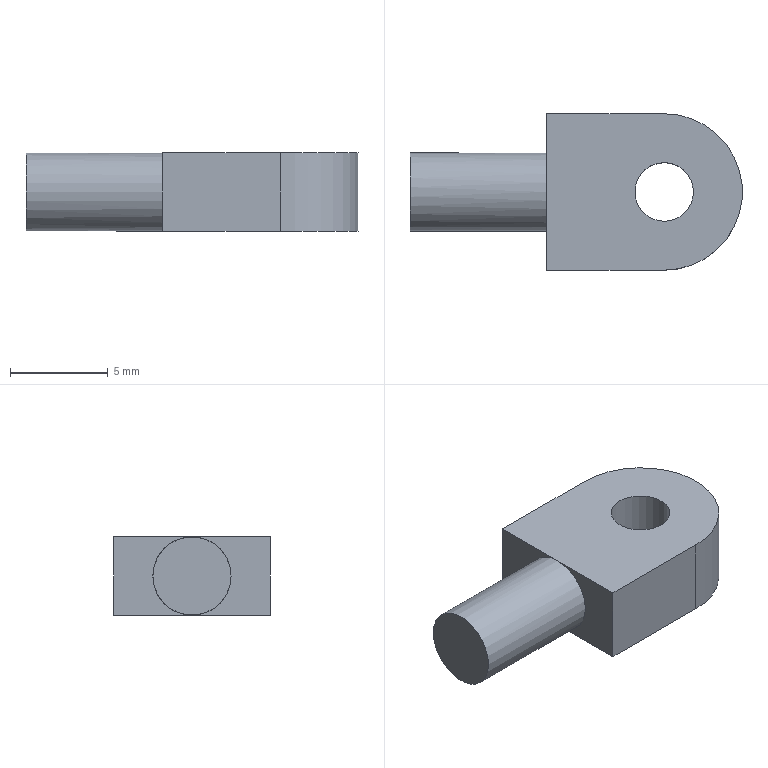Part | STEP file | 1-53.4 | 1 solid | 10 faces | box 17 x 8 x 4 mm | volume 352.221 mm3 | plane 7 | cylinder 3 | commonest cylinder face diameters 3 x1 4 x1 8 x1
STEP:
#1=CARTESIAN_POINT('',(0.,0.,0.));
#2=DIRECTION('',(0.,0.,1.));
#3=DIRECTION('',(1.,0.,0.));
#4=AXIS2_PLACEMENT_3D('',#1,#2,#3);
#5=CARTESIAN_POINT('',(0.,-4.,-2.));
#6=VERTEX_POINT('',#5);
#7=CARTESIAN_POINT('',(0.,4.,-2.));
#8=VERTEX_POINT('',#7);
#9=CARTESIAN_POINT('',(0.,0.,-2.));
#10=DIRECTION('',(0.,0.,1.));
#11=DIRECTION('',(0.,-1.,0.));
#12=AXIS2_PLACEMENT_3D('',#9,#10,#11);
#13=CIRCLE('',#12,4.);
#14=CARTESIAN_POINT('',(-1.,1.,-2.));
#15=DIRECTION('',(0.,0.,1.));
#16=DIRECTION('',(0.,1.,0.));
#17=AXIS2_PLACEMENT_3D('',#14,#15,#16);
#18=PLANE('',#17);
#19=CARTESIAN_POINT('',(-1.,-1.));
#20=DIRECTION('',(-1.,0.));
#21=AXIS2_PLACEMENT_2D('',#19,#20);
#22=CIRCLE('',#21,4.);
#23=(GEOMETRIC_REPRESENTATION_CONTEXT(2)PARAMETRIC_REPRESENTATION_CONTEXT()REPRESENTATION_CONTEXT('',''));
#24=DEFINITIONAL_REPRESENTATION('',(#22),#23);
#25=PCURVE('',#18,#24);
#26=CARTESIAN_POINT('',(0.,0.,-2.));
#27=DIRECTION('',(0.,0.,1.));
#28=DIRECTION('',(0.,-1.,0.));
#29=AXIS2_PLACEMENT_3D('',#26,#27,#28);
#30=CYLINDRICAL_SURFACE('',#29,4.);
#31=CARTESIAN_POINT('',(0.,0.));
#32=DIRECTION('',(1.,0.));
#33=VECTOR('',#32,1.);
#34=LINE('',#31,#33);
#35=(GEOMETRIC_REPRESENTATION_CONTEXT(2)PARAMETRIC_REPRESENTATION_CONTEXT()REPRESENTATION_CONTEXT('',''));
#36=DEFINITIONAL_REPRESENTATION('',(#34),#35);
#37=PCURVE('',#30,#36);
#38=SURFACE_CURVE('',#13,(#25,#37),.PCURVE_S1.);
#39=EDGE_CURVE('',#6,#8,#38,.T.);
#40=ORIENTED_EDGE('',*,*,#39,.T.);
#41=CARTESIAN_POINT('',(-6.,4.,-2.));
#42=VERTEX_POINT('',#41);
#43=CARTESIAN_POINT('',(0.,4.,-2.));
#44=DIRECTION('',(-1.,0.,0.));
#45=VECTOR('',#44,1.);
#46=LINE('',#43,#45);
#47=CARTESIAN_POINT('',(3.,-1.));
#48=DIRECTION('',(0.,1.));
#49=VECTOR('',#48,1.);
#50=LINE('',#47,#49);
#51=(GEOMETRIC_REPRESENTATION_CONTEXT(2)PARAMETRIC_REPRESENTATION_CONTEXT()REPRESENTATION_CONTEXT('',''));
#52=DEFINITIONAL_REPRESENTATION('',(#50),#51);
#53=PCURVE('',#18,#52);
#54=CARTESIAN_POINT('',(-3.,4.,0.));
#55=DIRECTION('',(0.,1.,0.));
#56=DIRECTION('',(-1.,0.,0.));
#57=AXIS2_PLACEMENT_3D('',#54,#55,#56);
#58=PLANE('',#57);
#59=CARTESIAN_POINT('',(-3.,-2.));
#60=DIRECTION('',(1.,0.));
#61=VECTOR('',#60,1.);
#62=LINE('',#59,#61);
#63=(GEOMETRIC_REPRESENTATION_CONTEXT(2)PARAMETRIC_REPRESENTATION_CONTEXT()REPRESENTATION_CONTEXT('',''));
#64=DEFINITIONAL_REPRESENTATION('',(#62),#63);
#65=PCURVE('',#58,#64);
#66=SURFACE_CURVE('',#46,(#53,#65),.PCURVE_S1.);
#67=EDGE_CURVE('',#8,#42,#66,.T.);
#68=ORIENTED_EDGE('',*,*,#67,.T.);
#69=CARTESIAN_POINT('',(-6.,0.,-2.));
#70=VERTEX_POINT('',#69);
#71=CARTESIAN_POINT('',(-6.,4.,-2.));
#72=DIRECTION('',(0.,-1.,0.));
#73=VECTOR('',#72,1.);
#74=LINE('',#71,#73);
#75=CARTESIAN_POINT('',(3.,5.));
#76=DIRECTION('',(-1.,0.));
#77=VECTOR('',#76,1.);
#78=LINE('',#75,#77);
#79=(GEOMETRIC_REPRESENTATION_CONTEXT(2)PARAMETRIC_REPRESENTATION_CONTEXT()REPRESENTATION_CONTEXT('',''));
#80=DEFINITIONAL_REPRESENTATION('',(#78),#79);
#81=PCURVE('',#18,#80);
#82=CARTESIAN_POINT('',(-6.,0.,0.));
#83=DIRECTION('',(-1.,0.,0.));
#84=DIRECTION('',(0.,-1.,0.));
#85=AXIS2_PLACEMENT_3D('',#82,#83,#84);
#86=PLANE('',#85);
#87=CARTESIAN_POINT('',(-4.,-2.));
#88=DIRECTION('',(1.,0.));
#89=VECTOR('',#88,1.);
#90=LINE('',#87,#89);
#91=(GEOMETRIC_REPRESENTATION_CONTEXT(2)PARAMETRIC_REPRESENTATION_CONTEXT()REPRESENTATION_CONTEXT('',''));
#92=DEFINITIONAL_REPRESENTATION('',(#90),#91);
#93=PCURVE('',#86,#92);
#94=SURFACE_CURVE('',#74,(#81,#93),.PCURVE_S1.);
#95=EDGE_CURVE('',#42,#70,#94,.T.);
#96=ORIENTED_EDGE('',*,*,#95,.T.);
#97=CARTESIAN_POINT('',(-6.,-4.,-2.));
#98=VERTEX_POINT('',#97);
#99=CARTESIAN_POINT('',(-6.,0.,-2.));
#100=DIRECTION('',(0.,-1.,0.));
#101=VECTOR('',#100,1.);
#102=LINE('',#99,#101);
#103=CARTESIAN_POINT('',(-1.,5.));
#104=DIRECTION('',(-1.,0.));
#105=VECTOR('',#104,1.);
#106=LINE('',#103,#105);
#107=(GEOMETRIC_REPRESENTATION_CONTEXT(2)PARAMETRIC_REPRESENTATION_CONTEXT()REPRESENTATION_CONTEXT('',''));
#108=DEFINITIONAL_REPRESENTATION('',(#106),#107);
#109=PCURVE('',#18,#108);
#110=CARTESIAN_POINT('',(-6.,0.,0.));
#111=DIRECTION('',(-1.,0.,0.));
#112=DIRECTION('',(0.,-1.,0.));
#113=AXIS2_PLACEMENT_3D('',#110,#111,#112);
#114=PLANE('',#113);
#115=CARTESIAN_POINT('',(0.,-2.));
#116=DIRECTION('',(1.,0.));
#117=VECTOR('',#116,1.);
#118=LINE('',#115,#117);
#119=(GEOMETRIC_REPRESENTATION_CONTEXT(2)PARAMETRIC_REPRESENTATION_CONTEXT()REPRESENTATION_CONTEXT('',''));
#120=DEFINITIONAL_REPRESENTATION('',(#118),#119);
#121=PCURVE('',#114,#120);
#122=SURFACE_CURVE('',#102,(#109,#121),.PCURVE_S1.);
#123=EDGE_CURVE('',#70,#98,#122,.T.);
#124=ORIENTED_EDGE('',*,*,#123,.T.);
#125=CARTESIAN_POINT('',(-6.,-4.,-2.));
#126=DIRECTION('',(1.,0.,0.));
#127=VECTOR('',#126,1.);
#128=LINE('',#125,#127);
#129=CARTESIAN_POINT('',(-5.,5.));
#130=DIRECTION('',(0.,-1.));
#131=VECTOR('',#130,1.);
#132=LINE('',#129,#131);
#133=(GEOMETRIC_REPRESENTATION_CONTEXT(2)PARAMETRIC_REPRESENTATION_CONTEXT()REPRESENTATION_CONTEXT('',''));
#134=DEFINITIONAL_REPRESENTATION('',(#132),#133);
#135=PCURVE('',#18,#134);
#136=CARTESIAN_POINT('',(-3.,-4.,0.));
#137=DIRECTION('',(0.,-1.,0.));
#138=DIRECTION('',(1.,0.,0.));
#139=AXIS2_PLACEMENT_3D('',#136,#137,#138);
#140=PLANE('',#139);
#141=CARTESIAN_POINT('',(-3.,-2.));
#142=DIRECTION('',(1.,0.));
#143=VECTOR('',#142,1.);
#144=LINE('',#141,#143);
#145=(GEOMETRIC_REPRESENTATION_CONTEXT(2)PARAMETRIC_REPRESENTATION_CONTEXT()REPRESENTATION_CONTEXT('',''));
#146=DEFINITIONAL_REPRESENTATION('',(#144),#145);
#147=PCURVE('',#140,#146);
#148=SURFACE_CURVE('',#128,(#135,#147),.PCURVE_S1.);
#149=EDGE_CURVE('',#98,#6,#148,.T.);
#150=ORIENTED_EDGE('',*,*,#149,.T.);
#151=EDGE_LOOP('',(#40,#68,#96,#124,#150));
#152=FACE_BOUND('',#151,.F.);
#153=CARTESIAN_POINT('',(0.,1.5,-2.));
#154=VERTEX_POINT('',#153);
#155=CARTESIAN_POINT('',(0.,0.,-2.));
#156=DIRECTION('',(0.,0.,-1.));
#157=DIRECTION('',(0.,1.,0.));
#158=AXIS2_PLACEMENT_3D('',#155,#156,#157);
#159=CIRCLE('',#158,1.5);
#160=CARTESIAN_POINT('',(0.5,-1.));
#161=CARTESIAN_POINT('',(0.5,-3.598));
#162=CARTESIAN_POINT('',(-1.75,-2.299));
#163=CARTESIAN_POINT('',(-4.,-1.));
#164=CARTESIAN_POINT('',(-1.75,0.299));
#165=CARTESIAN_POINT('',(0.5,1.598));
#166=CARTESIAN_POINT('',(0.5,-1.));
#167=(BOUNDED_CURVE()B_SPLINE_CURVE(2,(#160,#161,#162,#163,#164,#165,#166),.UNSPECIFIED.,.T.,.F.)B_SPLINE_CURVE_WITH_KNOTS((1,2,2,2,2,1),(-2.094,0.,2.094,4.189,6.283,8.378),.UNSPECIFIED.)CURVE()GEOMETRIC_REPRESENTATION_ITEM()RATIONAL_B_SPLINE_CURVE((1.,0.5,1.,0.5,1.,0.5,1.))REPRESENTATION_ITEM(''));
#168=(GEOMETRIC_REPRESENTATION_CONTEXT(2)PARAMETRIC_REPRESENTATION_CONTEXT()REPRESENTATION_CONTEXT('',''));
#169=DEFINITIONAL_REPRESENTATION('',(#167),#168);
#170=PCURVE('',#18,#169);
#171=CARTESIAN_POINT('',(0.,0.,-2.));
#172=DIRECTION('',(0.,0.,1.));
#173=DIRECTION('',(0.,1.,0.));
#174=AXIS2_PLACEMENT_3D('',#171,#172,#173);
#175=CYLINDRICAL_SURFACE('',#174,1.5);
#176=CARTESIAN_POINT('',(6.283,0.));
#177=DIRECTION('',(-1.,0.));
#178=VECTOR('',#177,1.);
#179=LINE('',#176,#178);
#180=(GEOMETRIC_REPRESENTATION_CONTEXT(2)PARAMETRIC_REPRESENTATION_CONTEXT()REPRESENTATION_CONTEXT('',''));
#181=DEFINITIONAL_REPRESENTATION('',(#179),#180);
#182=PCURVE('',#175,#181);
#183=SURFACE_CURVE('',#159,(#170,#182),.PCURVE_S1.);
#184=EDGE_CURVE('',#154,#154,#183,.T.);
#185=ORIENTED_EDGE('',*,*,#184,.T.);
#186=EDGE_LOOP('',(#185));
#187=FACE_BOUND('',#186,.F.);
#188=ADVANCED_FACE('',(#152,#187),#18,.F.);
#189=CARTESIAN_POINT('',(0.,-4.,2.));
#190=VERTEX_POINT('',#189);
#191=CARTESIAN_POINT('',(0.,4.,2.));
#192=VERTEX_POINT('',#191);
#193=CARTESIAN_POINT('',(0.,0.,2.));
#194=DIRECTION('',(0.,0.,1.));
#195=DIRECTION('',(0.,-1.,0.));
#196=AXIS2_PLACEMENT_3D('',#193,#194,#195);
#197=CIRCLE('',#196,4.);
#198=CARTESIAN_POINT('',(-1.,1.,2.));
#199=DIRECTION('',(0.,0.,1.));
#200=DIRECTION('',(0.,1.,0.));
#201=AXIS2_PLACEMENT_3D('',#198,#199,#200);
#202=PLANE('',#201);
#203=CARTESIAN_POINT('',(-1.,-1.));
#204=DIRECTION('',(-1.,0.));
#205=AXIS2_PLACEMENT_2D('',#203,#204);
#206=CIRCLE('',#205,4.);
#207=(GEOMETRIC_REPRESENTATION_CONTEXT(2)PARAMETRIC_REPRESENTATION_CONTEXT()REPRESENTATION_CONTEXT('',''));
#208=DEFINITIONAL_REPRESENTATION('',(#206),#207);
#209=PCURVE('',#202,#208);
#210=CARTESIAN_POINT('',(0.,4.));
#211=DIRECTION('',(1.,0.));
#212=VECTOR('',#211,1.);
#213=LINE('',#210,#212);
#214=(GEOMETRIC_REPRESENTATION_CONTEXT(2)PARAMETRIC_REPRESENTATION_CONTEXT()REPRESENTATION_CONTEXT('',''));
#215=DEFINITIONAL_REPRESENTATION('',(#213),#214);
#216=PCURVE('',#30,#215);
#217=SURFACE_CURVE('',#197,(#209,#216),.PCURVE_S1.);
#218=EDGE_CURVE('',#190,#192,#217,.T.);
#219=ORIENTED_EDGE('',*,*,#218,.T.);
#220=CARTESIAN_POINT('',(-6.,4.,2.));
#221=VERTEX_POINT('',#220);
#222=CARTESIAN_POINT('',(0.,4.,2.));
#223=DIRECTION('',(-1.,0.,0.));
#224=VECTOR('',#223,1.);
#225=LINE('',#222,#224);
#226=CARTESIAN_POINT('',(3.,-1.));
#227=DIRECTION('',(0.,1.));
#228=VECTOR('',#227,1.);
#229=LINE('',#226,#228);
#230=(GEOMETRIC_REPRESENTATION_CONTEXT(2)PARAMETRIC_REPRESENTATION_CONTEXT()REPRESENTATION_CONTEXT('',''));
#231=DEFINITIONAL_REPRESENTATION('',(#229),#230);
#232=PCURVE('',#202,#231);
#233=CARTESIAN_POINT('',(-3.,2.));
#234=DIRECTION('',(1.,0.));
#235=VECTOR('',#234,1.);
#236=LINE('',#233,#235);
#237=(GEOMETRIC_REPRESENTATION_CONTEXT(2)PARAMETRIC_REPRESENTATION_CONTEXT()REPRESENTATION_CONTEXT('',''));
#238=DEFINITIONAL_REPRESENTATION('',(#236),#237);
#239=PCURVE('',#58,#238);
#240=SURFACE_CURVE('',#225,(#232,#239),.PCURVE_S1.);
#241=EDGE_CURVE('',#192,#221,#240,.T.);
#242=ORIENTED_EDGE('',*,*,#241,.T.);
#243=CARTESIAN_POINT('',(-6.,0.,2.));
#244=VERTEX_POINT('',#243);
#245=CARTESIAN_POINT('',(-6.,4.,2.));
#246=DIRECTION('',(0.,-1.,0.));
#247=VECTOR('',#246,1.);
#248=LINE('',#245,#247);
#249=CARTESIAN_POINT('',(3.,5.));
#250=DIRECTION('',(-1.,0.));
#251=VECTOR('',#250,1.);
#252=LINE('',#249,#251);
#253=(GEOMETRIC_REPRESENTATION_CONTEXT(2)PARAMETRIC_REPRESENTATION_CONTEXT()REPRESENTATION_CONTEXT('',''));
#254=DEFINITIONAL_REPRESENTATION('',(#252),#253);
#255=PCURVE('',#202,#254);
#256=CARTESIAN_POINT('',(-4.,2.));
#257=DIRECTION('',(1.,0.));
#258=VECTOR('',#257,1.);
#259=LINE('',#256,#258);
#260=(GEOMETRIC_REPRESENTATION_CONTEXT(2)PARAMETRIC_REPRESENTATION_CONTEXT()REPRESENTATION_CONTEXT('',''));
#261=DEFINITIONAL_REPRESENTATION('',(#259),#260);
#262=PCURVE('',#86,#261);
#263=SURFACE_CURVE('',#248,(#255,#262),.PCURVE_S1.);
#264=EDGE_CURVE('',#221,#244,#263,.T.);
#265=ORIENTED_EDGE('',*,*,#264,.T.);
#266=CARTESIAN_POINT('',(-6.,-4.,2.));
#267=VERTEX_POINT('',#266);
#268=CARTESIAN_POINT('',(-6.,0.,2.));
#269=DIRECTION('',(0.,-1.,0.));
#270=VECTOR('',#269,1.);
#271=LINE('',#268,#270);
#272=CARTESIAN_POINT('',(-1.,5.));
#273=DIRECTION('',(-1.,0.));
#274=VECTOR('',#273,1.);
#275=LINE('',#272,#274);
#276=(GEOMETRIC_REPRESENTATION_CONTEXT(2)PARAMETRIC_REPRESENTATION_CONTEXT()REPRESENTATION_CONTEXT('',''));
#277=DEFINITIONAL_REPRESENTATION('',(#275),#276);
#278=PCURVE('',#202,#277);
#279=CARTESIAN_POINT('',(0.,2.));
#280=DIRECTION('',(1.,0.));
#281=VECTOR('',#280,1.);
#282=LINE('',#279,#281);
#283=(GEOMETRIC_REPRESENTATION_CONTEXT(2)PARAMETRIC_REPRESENTATION_CONTEXT()REPRESENTATION_CONTEXT('',''));
#284=DEFINITIONAL_REPRESENTATION('',(#282),#283);
#285=PCURVE('',#114,#284);
#286=SURFACE_CURVE('',#271,(#278,#285),.PCURVE_S1.);
#287=EDGE_CURVE('',#244,#267,#286,.T.);
#288=ORIENTED_EDGE('',*,*,#287,.T.);
#289=CARTESIAN_POINT('',(-6.,-4.,2.));
#290=DIRECTION('',(1.,0.,0.));
#291=VECTOR('',#290,1.);
#292=LINE('',#289,#291);
#293=CARTESIAN_POINT('',(-5.,5.));
#294=DIRECTION('',(0.,-1.));
#295=VECTOR('',#294,1.);
#296=LINE('',#293,#295);
#297=(GEOMETRIC_REPRESENTATION_CONTEXT(2)PARAMETRIC_REPRESENTATION_CONTEXT()REPRESENTATION_CONTEXT('',''));
#298=DEFINITIONAL_REPRESENTATION('',(#296),#297);
#299=PCURVE('',#202,#298);
#300=CARTESIAN_POINT('',(-3.,2.));
#301=DIRECTION('',(1.,0.));
#302=VECTOR('',#301,1.);
#303=LINE('',#300,#302);
#304=(GEOMETRIC_REPRESENTATION_CONTEXT(2)PARAMETRIC_REPRESENTATION_CONTEXT()REPRESENTATION_CONTEXT('',''));
#305=DEFINITIONAL_REPRESENTATION('',(#303),#304);
#306=PCURVE('',#140,#305);
#307=SURFACE_CURVE('',#292,(#299,#306),.PCURVE_S1.);
#308=EDGE_CURVE('',#267,#190,#307,.T.);
#309=ORIENTED_EDGE('',*,*,#308,.T.);
#310=EDGE_LOOP('',(#219,#242,#265,#288,#309));
#311=FACE_BOUND('',#310,.T.);
#312=CARTESIAN_POINT('',(0.,1.5,2.));
#313=VERTEX_POINT('',#312);
#314=CARTESIAN_POINT('',(0.,0.,2.));
#315=DIRECTION('',(0.,0.,-1.));
#316=DIRECTION('',(0.,1.,0.));
#317=AXIS2_PLACEMENT_3D('',#314,#315,#316);
#318=CIRCLE('',#317,1.5);
#319=CARTESIAN_POINT('',(0.5,-1.));
#320=CARTESIAN_POINT('',(0.5,-3.598));
#321=CARTESIAN_POINT('',(-1.75,-2.299));
#322=CARTESIAN_POINT('',(-4.,-1.));
#323=CARTESIAN_POINT('',(-1.75,0.299));
#324=CARTESIAN_POINT('',(0.5,1.598));
#325=CARTESIAN_POINT('',(0.5,-1.));
#326=(BOUNDED_CURVE()B_SPLINE_CURVE(2,(#319,#320,#321,#322,#323,#324,#325),.UNSPECIFIED.,.T.,.F.)B_SPLINE_CURVE_WITH_KNOTS((1,2,2,2,2,1),(-2.094,0.,2.094,4.189,6.283,8.378),.UNSPECIFIED.)CURVE()GEOMETRIC_REPRESENTATION_ITEM()RATIONAL_B_SPLINE_CURVE((1.,0.5,1.,0.5,1.,0.5,1.))REPRESENTATION_ITEM(''));
#327=(GEOMETRIC_REPRESENTATION_CONTEXT(2)PARAMETRIC_REPRESENTATION_CONTEXT()REPRESENTATION_CONTEXT('',''));
#328=DEFINITIONAL_REPRESENTATION('',(#326),#327);
#329=PCURVE('',#202,#328);
#330=CARTESIAN_POINT('',(6.283,4.));
#331=DIRECTION('',(-1.,0.));
#332=VECTOR('',#331,1.);
#333=LINE('',#330,#332);
#334=(GEOMETRIC_REPRESENTATION_CONTEXT(2)PARAMETRIC_REPRESENTATION_CONTEXT()REPRESENTATION_CONTEXT('',''));
#335=DEFINITIONAL_REPRESENTATION('',(#333),#334);
#336=PCURVE('',#175,#335);
#337=SURFACE_CURVE('',#318,(#329,#336),.PCURVE_S1.);
#338=EDGE_CURVE('',#313,#313,#337,.T.);
#339=ORIENTED_EDGE('',*,*,#338,.T.);
#340=EDGE_LOOP('',(#339));
#341=FACE_BOUND('',#340,.T.);
#342=ADVANCED_FACE('',(#311,#341),#202,.T.);
#343=ORIENTED_EDGE('',*,*,#39,.T.);
#344=CARTESIAN_POINT('',(0.,4.,-2.));
#345=DIRECTION('',(0.,0.,1.));
#346=VECTOR('',#345,1.);
#347=LINE('',#344,#346);
#348=CARTESIAN_POINT('',(3.142,0.));
#349=DIRECTION('',(0.,1.));
#350=VECTOR('',#349,1.);
#351=LINE('',#348,#350);
#352=(GEOMETRIC_REPRESENTATION_CONTEXT(2)PARAMETRIC_REPRESENTATION_CONTEXT()REPRESENTATION_CONTEXT('',''));
#353=DEFINITIONAL_REPRESENTATION('',(#351),#352);
#354=PCURVE('',#30,#353);
#355=CARTESIAN_POINT('',(-3.,-2.));
#356=DIRECTION('',(0.,1.));
#357=VECTOR('',#356,1.);
#358=LINE('',#355,#357);
#359=(GEOMETRIC_REPRESENTATION_CONTEXT(2)PARAMETRIC_REPRESENTATION_CONTEXT()REPRESENTATION_CONTEXT('',''));
#360=DEFINITIONAL_REPRESENTATION('',(#358),#359);
#361=PCURVE('',#58,#360);
#362=SURFACE_CURVE('',#347,(#354,#361),.PCURVE_S1.);
#363=EDGE_CURVE('',#8,#192,#362,.T.);
#364=ORIENTED_EDGE('',*,*,#363,.T.);
#365=ORIENTED_EDGE('',*,*,#218,.F.);
#366=CARTESIAN_POINT('',(0.,-4.,-2.));
#367=DIRECTION('',(0.,0.,1.));
#368=VECTOR('',#367,1.);
#369=LINE('',#366,#368);
#370=CARTESIAN_POINT('',(0.,0.));
#371=DIRECTION('',(0.,1.));
#372=VECTOR('',#371,1.);
#373=LINE('',#370,#372);
#374=(GEOMETRIC_REPRESENTATION_CONTEXT(2)PARAMETRIC_REPRESENTATION_CONTEXT()REPRESENTATION_CONTEXT('',''));
#375=DEFINITIONAL_REPRESENTATION('',(#373),#374);
#376=PCURVE('',#30,#375);
#377=CARTESIAN_POINT('',(3.,-2.));
#378=DIRECTION('',(0.,1.));
#379=VECTOR('',#378,1.);
#380=LINE('',#377,#379);
#381=(GEOMETRIC_REPRESENTATION_CONTEXT(2)PARAMETRIC_REPRESENTATION_CONTEXT()REPRESENTATION_CONTEXT('',''));
#382=DEFINITIONAL_REPRESENTATION('',(#380),#381);
#383=PCURVE('',#140,#382);
#384=SURFACE_CURVE('',#369,(#376,#383),.PCURVE_S1.);
#385=EDGE_CURVE('',#6,#190,#384,.T.);
#386=ORIENTED_EDGE('',*,*,#385,.F.);
#387=EDGE_LOOP('',(#343,#364,#365,#386));
#388=FACE_BOUND('',#387,.T.);
#389=ADVANCED_FACE('',(#388),#30,.T.);
#390=ORIENTED_EDGE('',*,*,#67,.T.);
#391=CARTESIAN_POINT('',(-6.,4.,-2.));
#392=DIRECTION('',(0.,0.,1.));
#393=VECTOR('',#392,1.);
#394=LINE('',#391,#393);
#395=CARTESIAN_POINT('',(3.,-2.));
#396=DIRECTION('',(0.,1.));
#397=VECTOR('',#396,1.);
#398=LINE('',#395,#397);
#399=(GEOMETRIC_REPRESENTATION_CONTEXT(2)PARAMETRIC_REPRESENTATION_CONTEXT()REPRESENTATION_CONTEXT('',''));
#400=DEFINITIONAL_REPRESENTATION('',(#398),#399);
#401=PCURVE('',#58,#400);
#402=CARTESIAN_POINT('',(-4.,-2.));
#403=DIRECTION('',(0.,1.));
#404=VECTOR('',#403,1.);
#405=LINE('',#402,#404);
#406=(GEOMETRIC_REPRESENTATION_CONTEXT(2)PARAMETRIC_REPRESENTATION_CONTEXT()REPRESENTATION_CONTEXT('',''));
#407=DEFINITIONAL_REPRESENTATION('',(#405),#406);
#408=PCURVE('',#86,#407);
#409=SURFACE_CURVE('',#394,(#401,#408),.PCURVE_S1.);
#410=EDGE_CURVE('',#42,#221,#409,.T.);
#411=ORIENTED_EDGE('',*,*,#410,.T.);
#412=ORIENTED_EDGE('',*,*,#241,.F.);
#413=ORIENTED_EDGE('',*,*,#363,.F.);
#414=EDGE_LOOP('',(#390,#411,#412,#413));
#415=FACE_BOUND('',#414,.T.);
#416=ADVANCED_FACE('',(#415),#58,.T.);
#417=ORIENTED_EDGE('',*,*,#149,.T.);
#418=ORIENTED_EDGE('',*,*,#385,.T.);
#419=ORIENTED_EDGE('',*,*,#308,.F.);
#420=CARTESIAN_POINT('',(-6.,-4.,-2.));
#421=DIRECTION('',(0.,0.,1.));
#422=VECTOR('',#421,1.);
#423=LINE('',#420,#422);
#424=CARTESIAN_POINT('',(-3.,-2.));
#425=DIRECTION('',(0.,1.));
#426=VECTOR('',#425,1.);
#427=LINE('',#424,#426);
#428=(GEOMETRIC_REPRESENTATION_CONTEXT(2)PARAMETRIC_REPRESENTATION_CONTEXT()REPRESENTATION_CONTEXT('',''));
#429=DEFINITIONAL_REPRESENTATION('',(#427),#428);
#430=PCURVE('',#140,#429);
#431=CARTESIAN_POINT('',(4.,-2.));
#432=DIRECTION('',(0.,1.));
#433=VECTOR('',#432,1.);
#434=LINE('',#431,#433);
#435=(GEOMETRIC_REPRESENTATION_CONTEXT(2)PARAMETRIC_REPRESENTATION_CONTEXT()REPRESENTATION_CONTEXT('',''));
#436=DEFINITIONAL_REPRESENTATION('',(#434),#435);
#437=PCURVE('',#114,#436);
#438=SURFACE_CURVE('',#423,(#430,#437),.PCURVE_S1.);
#439=EDGE_CURVE('',#98,#267,#438,.T.);
#440=ORIENTED_EDGE('',*,*,#439,.F.);
#441=EDGE_LOOP('',(#417,#418,#419,#440));
#442=FACE_BOUND('',#441,.T.);
#443=ADVANCED_FACE('',(#442),#140,.T.);
#444=CARTESIAN_POINT('',(0.,1.5,-2.));
#445=DIRECTION('',(0.,0.,1.));
#446=VECTOR('',#445,1.);
#447=LINE('',#444,#446);
#448=CARTESIAN_POINT('',(6.283,0.));
#449=DIRECTION('',(0.,1.));
#450=VECTOR('',#449,1.);
#451=LINE('',#448,#450);
#452=(GEOMETRIC_REPRESENTATION_CONTEXT(2)PARAMETRIC_REPRESENTATION_CONTEXT()REPRESENTATION_CONTEXT('',''));
#453=DEFINITIONAL_REPRESENTATION('',(#451),#452);
#454=PCURVE('',#175,#453);
#455=CARTESIAN_POINT('',(0.,0.));
#456=DIRECTION('',(0.,1.));
#457=VECTOR('',#456,1.);
#458=LINE('',#455,#457);
#459=(GEOMETRIC_REPRESENTATION_CONTEXT(2)PARAMETRIC_REPRESENTATION_CONTEXT()REPRESENTATION_CONTEXT('',''));
#460=DEFINITIONAL_REPRESENTATION('',(#458),#459);
#461=PCURVE('',#175,#460);
#462=SEAM_CURVE('',#447,(#454,#461),.PCURVE_S1.);
#463=EDGE_CURVE('',#154,#313,#462,.T.);
#464=ORIENTED_EDGE('',*,*,#463,.T.);
#465=ORIENTED_EDGE('',*,*,#338,.T.);
#466=ORIENTED_EDGE('',*,*,#463,.F.);
#467=ORIENTED_EDGE('',*,*,#184,.F.);
#468=EDGE_LOOP('',(#464,#465,#466,#467));
#469=FACE_BOUND('',#468,.F.);
#470=ADVANCED_FACE('',(#469),#175,.F.);
#471=ORIENTED_EDGE('',*,*,#287,.F.);
#472=CARTESIAN_POINT('',(-6.,-2.,0.));
#473=VERTEX_POINT('',#472);
#474=CARTESIAN_POINT('',(-6.,0.,0.));
#475=DIRECTION('',(-1.,0.,0.));
#476=DIRECTION('',(0.,-1.,0.));
#477=AXIS2_PLACEMENT_3D('',#474,#475,#476);
#478=CIRCLE('',#477,2.);
#479=CARTESIAN_POINT('',(0.,0.));
#480=DIRECTION('',(1.,0.));
#481=AXIS2_PLACEMENT_2D('',#479,#480);
#482=CIRCLE('',#481,2.);
#483=(GEOMETRIC_REPRESENTATION_CONTEXT(2)PARAMETRIC_REPRESENTATION_CONTEXT()REPRESENTATION_CONTEXT('',''));
#484=DEFINITIONAL_REPRESENTATION('',(#482),#483);
#485=PCURVE('',#114,#484);
#486=CARTESIAN_POINT('',(-6.,0.,0.));
#487=DIRECTION('',(-1.,0.,0.));
#488=DIRECTION('',(0.,-1.,0.));
#489=AXIS2_PLACEMENT_3D('',#486,#487,#488);
#490=CYLINDRICAL_SURFACE('',#489,2.);
#491=CARTESIAN_POINT('',(0.,0.));
#492=DIRECTION('',(1.,0.));
#493=VECTOR('',#492,1.);
#494=LINE('',#491,#493);
#495=(GEOMETRIC_REPRESENTATION_CONTEXT(2)PARAMETRIC_REPRESENTATION_CONTEXT()REPRESENTATION_CONTEXT('',''));
#496=DEFINITIONAL_REPRESENTATION('',(#494),#495);
#497=PCURVE('',#490,#496);
#498=SURFACE_CURVE('',#478,(#485,#497),.PCURVE_S1.);
#499=EDGE_CURVE('',#473,#244,#498,.T.);
#500=ORIENTED_EDGE('',*,*,#499,.F.);
#501=CARTESIAN_POINT('',(-6.,0.,0.));
#502=DIRECTION('',(-1.,0.,0.));
#503=DIRECTION('',(0.,0.,-1.));
#504=AXIS2_PLACEMENT_3D('',#501,#502,#503);
#505=CIRCLE('',#504,2.);
#506=CARTESIAN_POINT('',(0.,0.));
#507=DIRECTION('',(0.,-1.));
#508=AXIS2_PLACEMENT_2D('',#506,#507);
#509=CIRCLE('',#508,2.);
#510=(GEOMETRIC_REPRESENTATION_CONTEXT(2)PARAMETRIC_REPRESENTATION_CONTEXT()REPRESENTATION_CONTEXT('',''));
#511=DEFINITIONAL_REPRESENTATION('',(#509),#510);
#512=PCURVE('',#114,#511);
#513=CARTESIAN_POINT('',(4.712,0.));
#514=DIRECTION('',(1.,0.));
#515=VECTOR('',#514,1.);
#516=LINE('',#513,#515);
#517=(GEOMETRIC_REPRESENTATION_CONTEXT(2)PARAMETRIC_REPRESENTATION_CONTEXT()REPRESENTATION_CONTEXT('',''));
#518=DEFINITIONAL_REPRESENTATION('',(#516),#517);
#519=PCURVE('',#490,#518);
#520=SURFACE_CURVE('',#505,(#512,#519),.PCURVE_S1.);
#521=EDGE_CURVE('',#70,#473,#520,.T.);
#522=ORIENTED_EDGE('',*,*,#521,.F.);
#523=ORIENTED_EDGE('',*,*,#123,.T.);
#524=ORIENTED_EDGE('',*,*,#439,.T.);
#525=EDGE_LOOP('',(#471,#500,#522,#523,#524));
#526=FACE_BOUND('',#525,.T.);
#527=ADVANCED_FACE('',(#526),#114,.T.);
#528=ORIENTED_EDGE('',*,*,#95,.T.);
#529=CARTESIAN_POINT('',(-6.,0.,0.));
#530=DIRECTION('',(-1.,0.,0.));
#531=DIRECTION('',(0.,0.,1.));
#532=AXIS2_PLACEMENT_3D('',#529,#530,#531);
#533=CIRCLE('',#532,2.);
#534=CARTESIAN_POINT('',(0.,0.));
#535=DIRECTION('',(0.,1.));
#536=AXIS2_PLACEMENT_2D('',#534,#535);
#537=CIRCLE('',#536,2.);
#538=(GEOMETRIC_REPRESENTATION_CONTEXT(2)PARAMETRIC_REPRESENTATION_CONTEXT()REPRESENTATION_CONTEXT('',''));
#539=DEFINITIONAL_REPRESENTATION('',(#537),#538);
#540=PCURVE('',#86,#539);
#541=CARTESIAN_POINT('',(1.571,0.));
#542=DIRECTION('',(1.,0.));
#543=VECTOR('',#542,1.);
#544=LINE('',#541,#543);
#545=(GEOMETRIC_REPRESENTATION_CONTEXT(2)PARAMETRIC_REPRESENTATION_CONTEXT()REPRESENTATION_CONTEXT('',''));
#546=DEFINITIONAL_REPRESENTATION('',(#544),#545);
#547=PCURVE('',#490,#546);
#548=SURFACE_CURVE('',#533,(#540,#547),.PCURVE_S1.);
#549=EDGE_CURVE('',#244,#70,#548,.T.);
#550=ORIENTED_EDGE('',*,*,#549,.F.);
#551=ORIENTED_EDGE('',*,*,#264,.F.);
#552=ORIENTED_EDGE('',*,*,#410,.F.);
#553=EDGE_LOOP('',(#528,#550,#551,#552));
#554=FACE_BOUND('',#553,.T.);
#555=ADVANCED_FACE('',(#554),#86,.T.);
#556=ORIENTED_EDGE('',*,*,#499,.T.);
#557=ORIENTED_EDGE('',*,*,#549,.T.);
#558=ORIENTED_EDGE('',*,*,#521,.T.);
#559=CARTESIAN_POINT('',(-13.,-2.,0.));
#560=VERTEX_POINT('',#559);
#561=CARTESIAN_POINT('',(-6.,-2.,0.));
#562=DIRECTION('',(-1.,0.,0.));
#563=VECTOR('',#562,1.);
#564=LINE('',#561,#563);
#565=CARTESIAN_POINT('',(6.283,0.));
#566=DIRECTION('',(0.,1.));
#567=VECTOR('',#566,1.);
#568=LINE('',#565,#567);
#569=(GEOMETRIC_REPRESENTATION_CONTEXT(2)PARAMETRIC_REPRESENTATION_CONTEXT()REPRESENTATION_CONTEXT('',''));
#570=DEFINITIONAL_REPRESENTATION('',(#568),#569);
#571=PCURVE('',#490,#570);
#572=CARTESIAN_POINT('',(0.,0.));
#573=DIRECTION('',(0.,1.));
#574=VECTOR('',#573,1.);
#575=LINE('',#572,#574);
#576=(GEOMETRIC_REPRESENTATION_CONTEXT(2)PARAMETRIC_REPRESENTATION_CONTEXT()REPRESENTATION_CONTEXT('',''));
#577=DEFINITIONAL_REPRESENTATION('',(#575),#576);
#578=PCURVE('',#490,#577);
#579=SEAM_CURVE('',#564,(#571,#578),.PCURVE_S1.);
#580=EDGE_CURVE('',#473,#560,#579,.T.);
#581=ORIENTED_EDGE('',*,*,#580,.T.);
#582=CARTESIAN_POINT('',(-13.,0.,0.));
#583=DIRECTION('',(-1.,0.,0.));
#584=DIRECTION('',(0.,-1.,0.));
#585=AXIS2_PLACEMENT_3D('',#582,#583,#584);
#586=CIRCLE('',#585,2.);
#587=CARTESIAN_POINT('',(0.,7.));
#588=DIRECTION('',(1.,0.));
#589=VECTOR('',#588,1.);
#590=LINE('',#587,#589);
#591=(GEOMETRIC_REPRESENTATION_CONTEXT(2)PARAMETRIC_REPRESENTATION_CONTEXT()REPRESENTATION_CONTEXT('',''));
#592=DEFINITIONAL_REPRESENTATION('',(#590),#591);
#593=PCURVE('',#490,#592);
#594=CARTESIAN_POINT('',(-13.,0.5359,0.));
#595=DIRECTION('',(-1.,0.,0.));
#596=DIRECTION('',(0.,-1.,0.));
#597=AXIS2_PLACEMENT_3D('',#594,#595,#596);
#598=PLANE('',#597);
#599=CARTESIAN_POINT('',(0.5359,0.));
#600=DIRECTION('',(1.,0.));
#601=AXIS2_PLACEMENT_2D('',#599,#600);
#602=CIRCLE('',#601,2.);
#603=(GEOMETRIC_REPRESENTATION_CONTEXT(2)PARAMETRIC_REPRESENTATION_CONTEXT()REPRESENTATION_CONTEXT('',''));
#604=DEFINITIONAL_REPRESENTATION('',(#602),#603);
#605=PCURVE('',#598,#604);
#606=SURFACE_CURVE('',#586,(#593,#605),.PCURVE_S1.);
#607=EDGE_CURVE('',#560,#560,#606,.T.);
#608=ORIENTED_EDGE('',*,*,#607,.F.);
#609=ORIENTED_EDGE('',*,*,#580,.F.);
#610=EDGE_LOOP('',(#556,#557,#558,#581,#608,#609));
#611=FACE_BOUND('',#610,.T.);
#612=ADVANCED_FACE('',(#611),#490,.T.);
#613=ORIENTED_EDGE('',*,*,#607,.T.);
#614=EDGE_LOOP('',(#613));
#615=FACE_BOUND('',#614,.T.);
#616=ADVANCED_FACE('',(#615),#598,.T.);
#617=CLOSED_SHELL('',(#188,#342,#389,#416,#443,#470,#527,#555,#612,#616));
#618=MANIFOLD_SOLID_BREP('',#617);
#619=(LENGTH_UNIT()NAMED_UNIT(*)SI_UNIT(.MILLI.,.METRE.));
#620=UNCERTAINTY_MEASURE_WITH_UNIT(LENGTH_MEASURE(0.0000001),#619,'','');
#621=(NAMED_UNIT(*)PLANE_ANGLE_UNIT()SI_UNIT($,.RADIAN.));
#622=(NAMED_UNIT(*)SI_UNIT($,.STERADIAN.)SOLID_ANGLE_UNIT());
#623=(GEOMETRIC_REPRESENTATION_CONTEXT(3)GLOBAL_UNCERTAINTY_ASSIGNED_CONTEXT((#620))GLOBAL_UNIT_ASSIGNED_CONTEXT((#619,#621,#622))REPRESENTATION_CONTEXT('',''));
#624=ADVANCED_BREP_SHAPE_REPRESENTATION('',(#4,#618),#623);